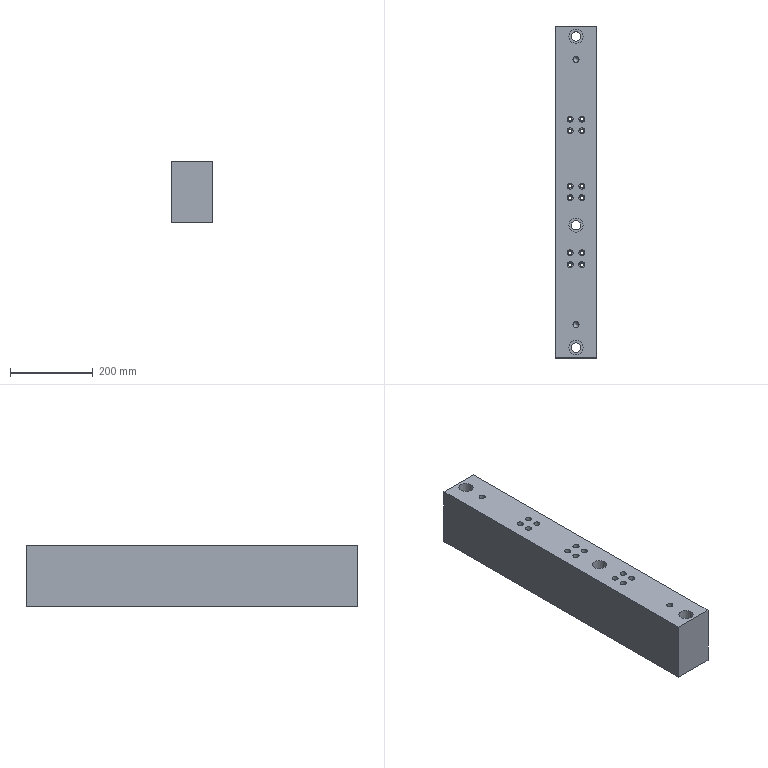Part | STEP file | lll_id2334_x_t | 1 solid | 61 faces | box 100 x 800 x 147.5 mm | volume 9817193 mm3 | cylinder 35 | plane 24 | cone 2 | commonest cylinder face diameters 9.009 x12 14.508 x12 23.009 x3 34.008 x3 80 x3 14.506 x2
STEP:
#1=CARTESIAN_POINT('',(2711.888,175.408,370.));
#2=VERTEX_POINT('',#1);
#3=CARTESIAN_POINT('',(2719.142,175.408,370.));
#4=DIRECTION('',(0.,0.,1.));
#5=DIRECTION('',(-1.,0.,0.));
#6=AXIS2_PLACEMENT_3D('',#3,#4,#5);
#7=CIRCLE('',#6,7.254);
#8=EDGE_CURVE('',#2,#2,#7,.T.);
#9=ORIENTED_EDGE('',*,*,#8,.F.);
#10=EDGE_LOOP('',(#9));
#11=FACE_BOUND('',#10,.T.);
#12=CARTESIAN_POINT('',(2711.888,147.124,370.));
#13=VERTEX_POINT('',#12);
#14=CARTESIAN_POINT('',(2719.142,147.124,370.));
#15=DIRECTION('',(0.,0.,1.));
#16=DIRECTION('',(-1.,0.,0.));
#17=AXIS2_PLACEMENT_3D('',#14,#15,#16);
#18=CIRCLE('',#17,7.254);
#19=EDGE_CURVE('',#13,#13,#18,.T.);
#20=ORIENTED_EDGE('',*,*,#19,.F.);
#21=EDGE_LOOP('',(#20));
#22=FACE_BOUND('',#21,.T.);
#23=CARTESIAN_POINT('',(2683.604,147.124,370.));
#24=VERTEX_POINT('',#23);
#25=CARTESIAN_POINT('',(2690.858,147.124,370.));
#26=DIRECTION('',(0.,0.,1.));
#27=DIRECTION('',(-1.,0.,0.));
#28=AXIS2_PLACEMENT_3D('',#25,#26,#27);
#29=CIRCLE('',#28,7.254);
#30=EDGE_CURVE('',#24,#24,#29,.T.);
#31=ORIENTED_EDGE('',*,*,#30,.F.);
#32=EDGE_LOOP('',(#31));
#33=FACE_BOUND('',#32,.T.);
#34=CARTESIAN_POINT('',(2683.604,14.142,370.));
#35=VERTEX_POINT('',#34);
#36=CARTESIAN_POINT('',(2690.858,14.142,370.));
#37=DIRECTION('',(0.,0.,1.));
#38=DIRECTION('',(-1.,0.,0.));
#39=AXIS2_PLACEMENT_3D('',#36,#37,#38);
#40=CIRCLE('',#39,7.254);
#41=EDGE_CURVE('',#35,#35,#40,.T.);
#42=ORIENTED_EDGE('',*,*,#41,.F.);
#43=EDGE_LOOP('',(#42));
#44=FACE_BOUND('',#43,.T.);
#45=CARTESIAN_POINT('',(2711.888,14.142,370.));
#46=VERTEX_POINT('',#45);
#47=CARTESIAN_POINT('',(2719.142,14.142,370.));
#48=DIRECTION('',(0.,0.,1.));
#49=DIRECTION('',(-1.,0.,0.));
#50=AXIS2_PLACEMENT_3D('',#47,#48,#49);
#51=CIRCLE('',#50,7.254);
#52=EDGE_CURVE('',#46,#46,#51,.T.);
#53=ORIENTED_EDGE('',*,*,#52,.F.);
#54=EDGE_LOOP('',(#53));
#55=FACE_BOUND('',#54,.T.);
#56=CARTESIAN_POINT('',(2711.888,-14.142,370.));
#57=VERTEX_POINT('',#56);
#58=CARTESIAN_POINT('',(2719.142,-14.142,370.));
#59=DIRECTION('',(0.,0.,1.));
#60=DIRECTION('',(-1.,0.,0.));
#61=AXIS2_PLACEMENT_3D('',#58,#59,#60);
#62=CIRCLE('',#61,7.254);
#63=EDGE_CURVE('',#57,#57,#62,.T.);
#64=ORIENTED_EDGE('',*,*,#63,.F.);
#65=EDGE_LOOP('',(#64));
#66=FACE_BOUND('',#65,.T.);
#67=CARTESIAN_POINT('',(2683.604,-14.142,370.));
#68=VERTEX_POINT('',#67);
#69=CARTESIAN_POINT('',(2690.858,-14.142,370.));
#70=DIRECTION('',(0.,0.,1.));
#71=DIRECTION('',(-1.,0.,0.));
#72=AXIS2_PLACEMENT_3D('',#69,#70,#71);
#73=CIRCLE('',#72,7.254);
#74=EDGE_CURVE('',#68,#68,#73,.T.);
#75=ORIENTED_EDGE('',*,*,#74,.F.);
#76=EDGE_LOOP('',(#75));
#77=FACE_BOUND('',#76,.T.);
#78=CARTESIAN_POINT('',(2711.888,-175.408,370.));
#79=VERTEX_POINT('',#78);
#80=CARTESIAN_POINT('',(2719.142,-175.408,370.));
#81=DIRECTION('',(0.,0.,1.));
#82=DIRECTION('',(-1.,0.,0.));
#83=AXIS2_PLACEMENT_3D('',#80,#81,#82);
#84=CIRCLE('',#83,7.254);
#85=EDGE_CURVE('',#79,#79,#84,.T.);
#86=ORIENTED_EDGE('',*,*,#85,.F.);
#87=EDGE_LOOP('',(#86));
#88=FACE_BOUND('',#87,.T.);
#89=CARTESIAN_POINT('',(2683.604,-175.408,370.));
#90=VERTEX_POINT('',#89);
#91=CARTESIAN_POINT('',(2690.858,-175.408,370.));
#92=DIRECTION('',(0.,0.,1.));
#93=DIRECTION('',(-1.,0.,0.));
#94=AXIS2_PLACEMENT_3D('',#91,#92,#93);
#95=CIRCLE('',#94,7.254);
#96=EDGE_CURVE('',#90,#90,#95,.T.);
#97=ORIENTED_EDGE('',*,*,#96,.F.);
#98=EDGE_LOOP('',(#97));
#99=FACE_BOUND('',#98,.T.);
#100=CARTESIAN_POINT('',(2683.604,-147.124,370.));
#101=VERTEX_POINT('',#100);
#102=CARTESIAN_POINT('',(2690.858,-147.124,370.));
#103=DIRECTION('',(0.,0.,1.));
#104=DIRECTION('',(-1.,0.,0.));
#105=AXIS2_PLACEMENT_3D('',#102,#103,#104);
#106=CIRCLE('',#105,7.254);
#107=EDGE_CURVE('',#101,#101,#106,.T.);
#108=ORIENTED_EDGE('',*,*,#107,.F.);
#109=EDGE_LOOP('',(#108));
#110=FACE_BOUND('',#109,.T.);
#111=CARTESIAN_POINT('',(2711.888,-147.124,370.));
#112=VERTEX_POINT('',#111);
#113=CARTESIAN_POINT('',(2719.142,-147.124,370.));
#114=DIRECTION('',(0.,0.,1.));
#115=DIRECTION('',(-1.,0.,0.));
#116=AXIS2_PLACEMENT_3D('',#113,#114,#115);
#117=CIRCLE('',#116,7.254);
#118=EDGE_CURVE('',#112,#112,#117,.T.);
#119=ORIENTED_EDGE('',*,*,#118,.F.);
#120=EDGE_LOOP('',(#119));
#121=FACE_BOUND('',#120,.T.);
#122=CARTESIAN_POINT('',(2683.604,175.408,370.));
#123=VERTEX_POINT('',#122);
#124=CARTESIAN_POINT('',(2690.858,175.408,370.));
#125=DIRECTION('',(0.,0.,1.));
#126=DIRECTION('',(-1.,0.,0.));
#127=AXIS2_PLACEMENT_3D('',#124,#125,#126);
#128=CIRCLE('',#127,7.254);
#129=EDGE_CURVE('',#123,#123,#128,.T.);
#130=ORIENTED_EDGE('',*,*,#129,.F.);
#131=EDGE_LOOP('',(#130));
#132=FACE_BOUND('',#131,.T.);
#133=CARTESIAN_POINT('',(2687.996,-80.,370.));
#134=VERTEX_POINT('',#133);
#135=CARTESIAN_POINT('',(2705.,-80.,370.));
#136=DIRECTION('',(0.,0.,-1.));
#137=DIRECTION('',(-1.,0.,0.));
#138=AXIS2_PLACEMENT_3D('',#135,#136,#137);
#139=CIRCLE('',#138,17.004);
#140=EDGE_CURVE('',#134,#134,#139,.T.);
#141=ORIENTED_EDGE('',*,*,#140,.T.);
#142=EDGE_LOOP('',(#141));
#143=FACE_BOUND('',#142,.T.);
#144=CARTESIAN_POINT('',(2755.,-400.,370.));
#145=VERTEX_POINT('',#144);
#146=CARTESIAN_POINT('',(2755.,400.,370.));
#147=VERTEX_POINT('',#146);
#148=CARTESIAN_POINT('',(2755.,600.,370.));
#149=DIRECTION('',(0.,1.,0.));
#150=VECTOR('',#149,1.);
#151=LINE('',#148,#150);
#152=EDGE_CURVE('',#145,#147,#151,.T.);
#153=ORIENTED_EDGE('',*,*,#152,.T.);
#154=CARTESIAN_POINT('',(2655.,400.,370.));
#155=VERTEX_POINT('',#154);
#156=CARTESIAN_POINT('',(2685.,400.,370.));
#157=DIRECTION('',(-1.,0.,0.));
#158=VECTOR('',#157,1.);
#159=LINE('',#156,#158);
#160=EDGE_CURVE('',#147,#155,#159,.T.);
#161=ORIENTED_EDGE('',*,*,#160,.T.);
#162=CARTESIAN_POINT('',(2655.,-400.,370.));
#163=VERTEX_POINT('',#162);
#164=CARTESIAN_POINT('',(2655.,0.,370.));
#165=DIRECTION('',(0.,1.,0.));
#166=VECTOR('',#165,1.);
#167=LINE('',#164,#166);
#168=EDGE_CURVE('',#163,#155,#167,.T.);
#169=ORIENTED_EDGE('',*,*,#168,.F.);
#170=CARTESIAN_POINT('',(2685.,-400.,370.));
#171=DIRECTION('',(1.,0.,0.));
#172=VECTOR('',#171,1.);
#173=LINE('',#170,#172);
#174=EDGE_CURVE('',#163,#145,#173,.T.);
#175=ORIENTED_EDGE('',*,*,#174,.T.);
#176=EDGE_LOOP('',(#153,#161,#169,#175));
#177=FACE_BOUND('',#176,.T.);
#178=CARTESIAN_POINT('',(2687.996,375.,370.));
#179=VERTEX_POINT('',#178);
#180=CARTESIAN_POINT('',(2705.,375.,370.));
#181=DIRECTION('',(0.,0.,-1.));
#182=DIRECTION('',(-1.,0.,0.));
#183=AXIS2_PLACEMENT_3D('',#180,#181,#182);
#184=CIRCLE('',#183,17.004);
#185=EDGE_CURVE('',#179,#179,#184,.T.);
#186=ORIENTED_EDGE('',*,*,#185,.T.);
#187=EDGE_LOOP('',(#186));
#188=FACE_BOUND('',#187,.T.);
#189=CARTESIAN_POINT('',(2687.996,-375.,370.));
#190=VERTEX_POINT('',#189);
#191=CARTESIAN_POINT('',(2705.,-375.,370.));
#192=DIRECTION('',(0.,0.,-1.));
#193=DIRECTION('',(-1.,0.,0.));
#194=AXIS2_PLACEMENT_3D('',#191,#192,#193);
#195=CIRCLE('',#194,17.004);
#196=EDGE_CURVE('',#190,#190,#195,.T.);
#197=ORIENTED_EDGE('',*,*,#196,.T.);
#198=EDGE_LOOP('',(#197));
#199=FACE_BOUND('',#198,.T.);
#200=CARTESIAN_POINT('',(2712.253,-320.,370.));
#201=VERTEX_POINT('',#200);
#202=CARTESIAN_POINT('',(2705.,-320.,370.));
#203=DIRECTION('',(0.,0.,-1.));
#204=DIRECTION('',(1.,0.,0.));
#205=AXIS2_PLACEMENT_3D('',#202,#203,#204);
#206=CIRCLE('',#205,7.253);
#207=EDGE_CURVE('',#201,#201,#206,.T.);
#208=ORIENTED_EDGE('',*,*,#207,.T.);
#209=EDGE_LOOP('',(#208));
#210=FACE_BOUND('',#209,.T.);
#211=CARTESIAN_POINT('',(2712.253,320.,370.));
#212=VERTEX_POINT('',#211);
#213=CARTESIAN_POINT('',(2705.,320.,370.));
#214=DIRECTION('',(0.,0.,1.));
#215=DIRECTION('',(1.,0.,0.));
#216=AXIS2_PLACEMENT_3D('',#213,#214,#215);
#217=CIRCLE('',#216,7.253);
#218=EDGE_CURVE('',#212,#212,#217,.T.);
#219=ORIENTED_EDGE('',*,*,#218,.F.);
#220=EDGE_LOOP('',(#219));
#221=FACE_BOUND('',#220,.T.);
#222=CARTESIAN_POINT('',(723.685,1.,370.));
#223=DIRECTION('',(0.,0.,-1.));
#224=DIRECTION('',(1.,0.,0.));
#225=AXIS2_PLACEMENT_3D('',#222,#223,#224);
#226=PLANE('',#225);
#227=ADVANCED_FACE('',(#11,#22,#33,#44,#55,#66,#77,#88,#99,#110,#121,#132,#143,#177,#188,#199,#210,#221),#226,.F.);
#228=CARTESIAN_POINT('',(2723.647,14.142,327.5));
#229=VERTEX_POINT('',#228);
#230=CARTESIAN_POINT('',(2719.142,14.142,327.5));
#231=DIRECTION('',(0.,0.,1.));
#232=DIRECTION('',(1.,0.,0.));
#233=AXIS2_PLACEMENT_3D('',#230,#231,#232);
#234=CIRCLE('',#233,4.505);
#235=EDGE_CURVE('',#229,#229,#234,.T.);
#236=ORIENTED_EDGE('',*,*,#235,.T.);
#237=EDGE_LOOP('',(#236));
#238=FACE_BOUND('',#237,.T.);
#239=CARTESIAN_POINT('',(2695.362,14.142,327.5));
#240=VERTEX_POINT('',#239);
#241=CARTESIAN_POINT('',(2690.858,14.142,327.5));
#242=DIRECTION('',(0.,0.,1.));
#243=DIRECTION('',(1.,0.,0.));
#244=AXIS2_PLACEMENT_3D('',#241,#242,#243);
#245=CIRCLE('',#244,4.505);
#246=EDGE_CURVE('',#240,#240,#245,.T.);
#247=ORIENTED_EDGE('',*,*,#246,.T.);
#248=EDGE_LOOP('',(#247));
#249=FACE_BOUND('',#248,.T.);
#250=CARTESIAN_POINT('',(2665.,0.,327.5));
#251=VERTEX_POINT('',#250);
#252=CARTESIAN_POINT('',(2705.,0.,327.5));
#253=DIRECTION('',(0.,0.,-1.));
#254=DIRECTION('',(-1.,0.,0.));
#255=AXIS2_PLACEMENT_3D('',#252,#253,#254);
#256=CIRCLE('',#255,40.);
#257=EDGE_CURVE('',#251,#251,#256,.T.);
#258=ORIENTED_EDGE('',*,*,#257,.T.);
#259=EDGE_LOOP('',(#258));
#260=FACE_BOUND('',#259,.T.);
#261=CARTESIAN_POINT('',(2695.362,-14.142,327.5));
#262=VERTEX_POINT('',#261);
#263=CARTESIAN_POINT('',(2690.858,-14.142,327.5));
#264=DIRECTION('',(0.,0.,1.));
#265=DIRECTION('',(1.,0.,0.));
#266=AXIS2_PLACEMENT_3D('',#263,#264,#265);
#267=CIRCLE('',#266,4.505);
#268=EDGE_CURVE('',#262,#262,#267,.T.);
#269=ORIENTED_EDGE('',*,*,#268,.T.);
#270=EDGE_LOOP('',(#269));
#271=FACE_BOUND('',#270,.T.);
#272=CARTESIAN_POINT('',(2723.647,-14.142,327.5));
#273=VERTEX_POINT('',#272);
#274=CARTESIAN_POINT('',(2719.142,-14.142,327.5));
#275=DIRECTION('',(0.,0.,1.));
#276=DIRECTION('',(1.,0.,0.));
#277=AXIS2_PLACEMENT_3D('',#274,#275,#276);
#278=CIRCLE('',#277,4.505);
#279=EDGE_CURVE('',#273,#273,#278,.T.);
#280=ORIENTED_EDGE('',*,*,#279,.T.);
#281=EDGE_LOOP('',(#280));
#282=FACE_BOUND('',#281,.T.);
#283=CARTESIAN_POINT('',(2705.,0.2078,327.5));
#284=DIRECTION('',(0.,0.,-1.));
#285=DIRECTION('',(-1.,0.,0.));
#286=AXIS2_PLACEMENT_3D('',#283,#284,#285);
#287=PLANE('',#286);
#288=ADVANCED_FACE('',(#238,#249,#260,#271,#282),#287,.T.);
#289=CARTESIAN_POINT('',(2723.647,-147.124,327.5));
#290=VERTEX_POINT('',#289);
#291=CARTESIAN_POINT('',(2719.142,-147.124,327.5));
#292=DIRECTION('',(0.,0.,1.));
#293=DIRECTION('',(1.,0.,0.));
#294=AXIS2_PLACEMENT_3D('',#291,#292,#293);
#295=CIRCLE('',#294,4.505);
#296=EDGE_CURVE('',#290,#290,#295,.T.);
#297=ORIENTED_EDGE('',*,*,#296,.T.);
#298=EDGE_LOOP('',(#297));
#299=FACE_BOUND('',#298,.T.);
#300=CARTESIAN_POINT('',(2695.362,-147.124,327.5));
#301=VERTEX_POINT('',#300);
#302=CARTESIAN_POINT('',(2690.858,-147.124,327.5));
#303=DIRECTION('',(0.,0.,1.));
#304=DIRECTION('',(1.,0.,0.));
#305=AXIS2_PLACEMENT_3D('',#302,#303,#304);
#306=CIRCLE('',#305,4.505);
#307=EDGE_CURVE('',#301,#301,#306,.T.);
#308=ORIENTED_EDGE('',*,*,#307,.T.);
#309=EDGE_LOOP('',(#308));
#310=FACE_BOUND('',#309,.T.);
#311=CARTESIAN_POINT('',(2665.,-161.266,327.5));
#312=VERTEX_POINT('',#311);
#313=CARTESIAN_POINT('',(2705.,-161.266,327.5));
#314=DIRECTION('',(0.,0.,-1.));
#315=DIRECTION('',(-1.,0.,0.));
#316=AXIS2_PLACEMENT_3D('',#313,#314,#315);
#317=CIRCLE('',#316,40.);
#318=EDGE_CURVE('',#312,#312,#317,.T.);
#319=ORIENTED_EDGE('',*,*,#318,.T.);
#320=EDGE_LOOP('',(#319));
#321=FACE_BOUND('',#320,.T.);
#322=CARTESIAN_POINT('',(2723.647,-175.408,327.5));
#323=VERTEX_POINT('',#322);
#324=CARTESIAN_POINT('',(2719.142,-175.408,327.5));
#325=DIRECTION('',(0.,0.,1.));
#326=DIRECTION('',(1.,0.,0.));
#327=AXIS2_PLACEMENT_3D('',#324,#325,#326);
#328=CIRCLE('',#327,4.505);
#329=EDGE_CURVE('',#323,#323,#328,.T.);
#330=ORIENTED_EDGE('',*,*,#329,.T.);
#331=EDGE_LOOP('',(#330));
#332=FACE_BOUND('',#331,.T.);
#333=CARTESIAN_POINT('',(2695.362,-175.408,327.5));
#334=VERTEX_POINT('',#333);
#335=CARTESIAN_POINT('',(2690.858,-175.408,327.5));
#336=DIRECTION('',(0.,0.,1.));
#337=DIRECTION('',(1.,0.,0.));
#338=AXIS2_PLACEMENT_3D('',#335,#336,#337);
#339=CIRCLE('',#338,4.505);
#340=EDGE_CURVE('',#334,#334,#339,.T.);
#341=ORIENTED_EDGE('',*,*,#340,.T.);
#342=EDGE_LOOP('',(#341));
#343=FACE_BOUND('',#342,.T.);
#344=CARTESIAN_POINT('',(2705.,-161.058,327.5));
#345=DIRECTION('',(0.,0.,-1.));
#346=DIRECTION('',(-1.,0.,0.));
#347=AXIS2_PLACEMENT_3D('',#344,#345,#346);
#348=PLANE('',#347);
#349=ADVANCED_FACE('',(#299,#310,#321,#332,#343),#348,.T.);
#350=CARTESIAN_POINT('',(2695.362,175.408,327.5));
#351=VERTEX_POINT('',#350);
#352=CARTESIAN_POINT('',(2690.858,175.408,327.5));
#353=DIRECTION('',(0.,0.,1.));
#354=DIRECTION('',(1.,0.,0.));
#355=AXIS2_PLACEMENT_3D('',#352,#353,#354);
#356=CIRCLE('',#355,4.505);
#357=EDGE_CURVE('',#351,#351,#356,.T.);
#358=ORIENTED_EDGE('',*,*,#357,.T.);
#359=EDGE_LOOP('',(#358));
#360=FACE_BOUND('',#359,.T.);
#361=CARTESIAN_POINT('',(2723.647,147.124,327.5));
#362=VERTEX_POINT('',#361);
#363=CARTESIAN_POINT('',(2719.142,147.124,327.5));
#364=DIRECTION('',(0.,0.,1.));
#365=DIRECTION('',(1.,0.,0.));
#366=AXIS2_PLACEMENT_3D('',#363,#364,#365);
#367=CIRCLE('',#366,4.505);
#368=EDGE_CURVE('',#362,#362,#367,.T.);
#369=ORIENTED_EDGE('',*,*,#368,.T.);
#370=EDGE_LOOP('',(#369));
#371=FACE_BOUND('',#370,.T.);
#372=CARTESIAN_POINT('',(2665.,161.266,327.5));
#373=VERTEX_POINT('',#372);
#374=CARTESIAN_POINT('',(2705.,161.266,327.5));
#375=DIRECTION('',(0.,0.,1.));
#376=DIRECTION('',(-1.,0.,0.));
#377=AXIS2_PLACEMENT_3D('',#374,#375,#376);
#378=CIRCLE('',#377,40.);
#379=EDGE_CURVE('',#373,#373,#378,.T.);
#380=ORIENTED_EDGE('',*,*,#379,.F.);
#381=EDGE_LOOP('',(#380));
#382=FACE_BOUND('',#381,.T.);
#383=CARTESIAN_POINT('',(2695.362,147.124,327.5));
#384=VERTEX_POINT('',#383);
#385=CARTESIAN_POINT('',(2690.858,147.124,327.5));
#386=DIRECTION('',(0.,0.,1.));
#387=DIRECTION('',(1.,0.,0.));
#388=AXIS2_PLACEMENT_3D('',#385,#386,#387);
#389=CIRCLE('',#388,4.505);
#390=EDGE_CURVE('',#384,#384,#389,.T.);
#391=ORIENTED_EDGE('',*,*,#390,.T.);
#392=EDGE_LOOP('',(#391));
#393=FACE_BOUND('',#392,.T.);
#394=CARTESIAN_POINT('',(2723.647,175.408,327.5));
#395=VERTEX_POINT('',#394);
#396=CARTESIAN_POINT('',(2719.142,175.408,327.5));
#397=DIRECTION('',(0.,0.,1.));
#398=DIRECTION('',(1.,0.,0.));
#399=AXIS2_PLACEMENT_3D('',#396,#397,#398);
#400=CIRCLE('',#399,4.505);
#401=EDGE_CURVE('',#395,#395,#400,.T.);
#402=ORIENTED_EDGE('',*,*,#401,.T.);
#403=EDGE_LOOP('',(#402));
#404=FACE_BOUND('',#403,.T.);
#405=CARTESIAN_POINT('',(2705.,161.474,327.5));
#406=DIRECTION('',(0.,0.,-1.));
#407=DIRECTION('',(-1.,0.,0.));
#408=AXIS2_PLACEMENT_3D('',#405,#406,#407);
#409=PLANE('',#408);
#410=ADVANCED_FACE('',(#360,#371,#382,#393,#404),#409,.T.);
#411=CARTESIAN_POINT('',(2693.495,-375.,222.5));
#412=VERTEX_POINT('',#411);
#413=CARTESIAN_POINT('',(2705.,-375.,222.5));
#414=DIRECTION('',(0.,0.,-1.));
#415=DIRECTION('',(-1.,0.,0.));
#416=AXIS2_PLACEMENT_3D('',#413,#414,#415);
#417=CIRCLE('',#416,11.505);
#418=EDGE_CURVE('',#412,#412,#417,.T.);
#419=ORIENTED_EDGE('',*,*,#418,.F.);
#420=EDGE_LOOP('',(#419));
#421=FACE_BOUND('',#420,.T.);
#422=CARTESIAN_POINT('',(2693.495,-80.,222.5));
#423=VERTEX_POINT('',#422);
#424=CARTESIAN_POINT('',(2705.,-80.,222.5));
#425=DIRECTION('',(0.,0.,-1.));
#426=DIRECTION('',(-1.,0.,0.));
#427=AXIS2_PLACEMENT_3D('',#424,#425,#426);
#428=CIRCLE('',#427,11.505);
#429=EDGE_CURVE('',#423,#423,#428,.T.);
#430=ORIENTED_EDGE('',*,*,#429,.F.);
#431=EDGE_LOOP('',(#430));
#432=FACE_BOUND('',#431,.T.);
#433=CARTESIAN_POINT('',(2693.495,375.,222.5));
#434=VERTEX_POINT('',#433);
#435=CARTESIAN_POINT('',(2705.,375.,222.5));
#436=DIRECTION('',(0.,0.,-1.));
#437=DIRECTION('',(-1.,0.,0.));
#438=AXIS2_PLACEMENT_3D('',#435,#436,#437);
#439=CIRCLE('',#438,11.505);
#440=EDGE_CURVE('',#434,#434,#439,.T.);
#441=ORIENTED_EDGE('',*,*,#440,.F.);
#442=EDGE_LOOP('',(#441));
#443=FACE_BOUND('',#442,.T.);
#444=CARTESIAN_POINT('',(2665.,-161.266,222.5));
#445=VERTEX_POINT('',#444);
#446=CARTESIAN_POINT('',(2705.,-161.266,222.5));
#447=DIRECTION('',(0.,0.,-1.));
#448=DIRECTION('',(-1.,0.,0.));
#449=AXIS2_PLACEMENT_3D('',#446,#447,#448);
#450=CIRCLE('',#449,40.);
#451=EDGE_CURVE('',#445,#445,#450,.T.);
#452=ORIENTED_EDGE('',*,*,#451,.F.);
#453=EDGE_LOOP('',(#452));
#454=FACE_BOUND('',#453,.T.);
#455=CARTESIAN_POINT('',(2665.,0.,222.5));
#456=VERTEX_POINT('',#455);
#457=CARTESIAN_POINT('',(2705.,0.,222.5));
#458=DIRECTION('',(0.,0.,-1.));
#459=DIRECTION('',(-1.,0.,0.));
#460=AXIS2_PLACEMENT_3D('',#457,#458,#459);
#461=CIRCLE('',#460,40.);
#462=EDGE_CURVE('',#456,#456,#461,.T.);
#463=ORIENTED_EDGE('',*,*,#462,.F.);
#464=EDGE_LOOP('',(#463));
#465=FACE_BOUND('',#464,.T.);
#466=CARTESIAN_POINT('',(2665.,161.266,222.5));
#467=VERTEX_POINT('',#466);
#468=CARTESIAN_POINT('',(2705.,161.266,222.5));
#469=DIRECTION('',(0.,0.,-1.));
#470=DIRECTION('',(-1.,0.,0.));
#471=AXIS2_PLACEMENT_3D('',#468,#469,#470);
#472=CIRCLE('',#471,40.);
#473=EDGE_CURVE('',#467,#467,#472,.T.);
#474=ORIENTED_EDGE('',*,*,#473,.F.);
#475=EDGE_LOOP('',(#474));
#476=FACE_BOUND('',#475,.T.);
#477=CARTESIAN_POINT('',(2755.,400.,222.5));
#478=VERTEX_POINT('',#477);
#479=CARTESIAN_POINT('',(2755.,-400.,222.5));
#480=VERTEX_POINT('',#479);
#481=CARTESIAN_POINT('',(2755.,1.,222.5));
#482=DIRECTION('',(0.,-1.,0.));
#483=VECTOR('',#482,1.);
#484=LINE('',#481,#483);
#485=EDGE_CURVE('',#478,#480,#484,.T.);
#486=ORIENTED_EDGE('',*,*,#485,.T.);
#487=CARTESIAN_POINT('',(2655.,-400.,222.5));
#488=VERTEX_POINT('',#487);
#489=CARTESIAN_POINT('',(4901.315,-400.,222.5));
#490=DIRECTION('',(-1.,0.,0.));
#491=VECTOR('',#490,1.);
#492=LINE('',#489,#491);
#493=EDGE_CURVE('',#480,#488,#492,.T.);
#494=ORIENTED_EDGE('',*,*,#493,.T.);
#495=CARTESIAN_POINT('',(2655.,400.,222.5));
#496=VERTEX_POINT('',#495);
#497=CARTESIAN_POINT('',(2655.,1.,222.5));
#498=DIRECTION('',(0.,-1.,0.));
#499=VECTOR('',#498,1.);
#500=LINE('',#497,#499);
#501=EDGE_CURVE('',#496,#488,#500,.T.);
#502=ORIENTED_EDGE('',*,*,#501,.F.);
#503=CARTESIAN_POINT('',(4901.315,400.,222.5));
#504=DIRECTION('',(1.,0.,0.));
#505=VECTOR('',#504,1.);
#506=LINE('',#503,#505);
#507=EDGE_CURVE('',#496,#478,#506,.T.);
#508=ORIENTED_EDGE('',*,*,#507,.T.);
#509=EDGE_LOOP('',(#486,#494,#502,#508));
#510=FACE_BOUND('',#509,.T.);
#511=CARTESIAN_POINT('',(4901.315,1.,222.5));
#512=DIRECTION('',(0.,0.,-1.));
#513=DIRECTION('',(-1.,0.,0.));
#514=AXIS2_PLACEMENT_3D('',#511,#512,#513);
#515=PLANE('',#514);
#516=ADVANCED_FACE('',(#421,#432,#443,#454,#465,#476,#510),#515,.T.);
#517=CARTESIAN_POINT('',(2755.,400.,291.25));
#518=DIRECTION('',(0.,0.,-1.));
#519=VECTOR('',#518,1.);
#520=LINE('',#517,#519);
#521=EDGE_CURVE('',#147,#478,#520,.T.);
#522=ORIENTED_EDGE('',*,*,#521,.F.);
#523=ORIENTED_EDGE('',*,*,#152,.F.);
#524=CARTESIAN_POINT('',(2755.,-400.,291.25));
#525=DIRECTION('',(0.,0.,1.));
#526=VECTOR('',#525,1.);
#527=LINE('',#524,#526);
#528=EDGE_CURVE('',#480,#145,#527,.T.);
#529=ORIENTED_EDGE('',*,*,#528,.F.);
#530=ORIENTED_EDGE('',*,*,#485,.F.);
#531=EDGE_LOOP('',(#522,#523,#529,#530));
#532=FACE_OUTER_BOUND('',#531,.T.);
#533=CARTESIAN_POINT('',(2755.,600.,360.));
#534=DIRECTION('',(1.,0.,0.));
#535=DIRECTION('',(0.,0.,-1.));
#536=AXIS2_PLACEMENT_3D('',#533,#534,#535);
#537=PLANE('',#536);
#538=ADVANCED_FACE('',(#532),#537,.T.);
#539=CARTESIAN_POINT('',(2655.,-400.,291.25));
#540=DIRECTION('',(0.,0.,-1.));
#541=VECTOR('',#540,1.);
#542=LINE('',#539,#541);
#543=EDGE_CURVE('',#163,#488,#542,.T.);
#544=ORIENTED_EDGE('',*,*,#543,.F.);
#545=ORIENTED_EDGE('',*,*,#168,.T.);
#546=CARTESIAN_POINT('',(2655.,400.,291.25));
#547=DIRECTION('',(0.,0.,-1.));
#548=VECTOR('',#547,1.);
#549=LINE('',#546,#548);
#550=EDGE_CURVE('',#155,#496,#549,.T.);
#551=ORIENTED_EDGE('',*,*,#550,.T.);
#552=ORIENTED_EDGE('',*,*,#501,.T.);
#553=EDGE_LOOP('',(#544,#545,#551,#552));
#554=FACE_OUTER_BOUND('',#553,.T.);
#555=CARTESIAN_POINT('',(2655.,0.,291.25));
#556=DIRECTION('',(1.,0.,0.));
#557=DIRECTION('',(0.,0.,-1.));
#558=AXIS2_PLACEMENT_3D('',#555,#556,#557);
#559=PLANE('',#558);
#560=ADVANCED_FACE('',(#554),#559,.F.);
#561=ORIENTED_EDGE('',*,*,#160,.F.);
#562=ORIENTED_EDGE('',*,*,#521,.T.);
#563=ORIENTED_EDGE('',*,*,#507,.F.);
#564=ORIENTED_EDGE('',*,*,#550,.F.);
#565=EDGE_LOOP('',(#561,#562,#563,#564));
#566=FACE_OUTER_BOUND('',#565,.T.);
#567=CARTESIAN_POINT('',(2685.,400.,291.25));
#568=DIRECTION('',(0.,1.,0.));
#569=DIRECTION('',(0.,0.,1.));
#570=AXIS2_PLACEMENT_3D('',#567,#568,#569);
#571=PLANE('',#570);
#572=ADVANCED_FACE('',(#566),#571,.T.);
#573=ORIENTED_EDGE('',*,*,#174,.F.);
#574=ORIENTED_EDGE('',*,*,#543,.T.);
#575=ORIENTED_EDGE('',*,*,#493,.F.);
#576=ORIENTED_EDGE('',*,*,#528,.T.);
#577=EDGE_LOOP('',(#573,#574,#575,#576));
#578=FACE_OUTER_BOUND('',#577,.T.);
#579=CARTESIAN_POINT('',(2685.,-400.,291.25));
#580=DIRECTION('',(0.,-1.,0.));
#581=DIRECTION('',(0.,0.,-1.));
#582=AXIS2_PLACEMENT_3D('',#579,#580,#581);
#583=PLANE('',#582);
#584=ADVANCED_FACE('',(#578),#583,.T.);
#585=ORIENTED_EDGE('',*,*,#379,.T.);
#586=EDGE_LOOP('',(#585));
#587=FACE_BOUND('',#586,.T.);
#588=ORIENTED_EDGE('',*,*,#473,.T.);
#589=EDGE_LOOP('',(#588));
#590=FACE_BOUND('',#589,.T.);
#591=CARTESIAN_POINT('',(2705.,161.266,346.5));
#592=DIRECTION('',(0.,0.,-1.));
#593=DIRECTION('',(1.,0.,0.));
#594=AXIS2_PLACEMENT_3D('',#591,#592,#593);
#595=CYLINDRICAL_SURFACE('',#594,40.);
#596=ADVANCED_FACE('',(#587,#590),#595,.F.);
#597=ORIENTED_EDGE('',*,*,#257,.F.);
#598=EDGE_LOOP('',(#597));
#599=FACE_BOUND('',#598,.T.);
#600=ORIENTED_EDGE('',*,*,#462,.T.);
#601=EDGE_LOOP('',(#600));
#602=FACE_BOUND('',#601,.T.);
#603=CARTESIAN_POINT('',(2705.,0.,181.5));
#604=DIRECTION('',(0.,0.,1.));
#605=DIRECTION('',(1.,0.,0.));
#606=AXIS2_PLACEMENT_3D('',#603,#604,#605);
#607=CYLINDRICAL_SURFACE('',#606,40.);
#608=ADVANCED_FACE('',(#599,#602),#607,.F.);
#609=ORIENTED_EDGE('',*,*,#318,.F.);
#610=EDGE_LOOP('',(#609));
#611=FACE_BOUND('',#610,.T.);
#612=ORIENTED_EDGE('',*,*,#451,.T.);
#613=EDGE_LOOP('',(#612));
#614=FACE_BOUND('',#613,.T.);
#615=CARTESIAN_POINT('',(2705.,-161.266,181.5));
#616=DIRECTION('',(0.,0.,1.));
#617=DIRECTION('',(1.,0.,0.));
#618=AXIS2_PLACEMENT_3D('',#615,#616,#617);
#619=CYLINDRICAL_SURFACE('',#618,40.);
#620=ADVANCED_FACE('',(#611,#614),#619,.F.);
#621=ORIENTED_EDGE('',*,*,#440,.T.);
#622=EDGE_LOOP('',(#621));
#623=FACE_BOUND('',#622,.T.);
#624=CARTESIAN_POINT('',(2693.495,375.,272.5));
#625=VERTEX_POINT('',#624);
#626=CARTESIAN_POINT('',(2705.,375.,272.5));
#627=DIRECTION('',(0.,0.,-1.));
#628=DIRECTION('',(-1.,0.,0.));
#629=AXIS2_PLACEMENT_3D('',#626,#627,#628);
#630=CIRCLE('',#629,11.505);
#631=EDGE_CURVE('',#625,#625,#630,.T.);
#632=ORIENTED_EDGE('',*,*,#631,.F.);
#633=EDGE_LOOP('',(#632));
#634=FACE_BOUND('',#633,.T.);
#635=CARTESIAN_POINT('',(2705.,375.,382.));
#636=DIRECTION('',(0.,0.,-1.));
#637=DIRECTION('',(1.,0.,0.));
#638=AXIS2_PLACEMENT_3D('',#635,#636,#637);
#639=CYLINDRICAL_SURFACE('',#638,11.505);
#640=ADVANCED_FACE('',(#623,#634),#639,.F.);
#641=ORIENTED_EDGE('',*,*,#631,.T.);
#642=EDGE_LOOP('',(#641));
#643=FACE_BOUND('',#642,.T.);
#644=CARTESIAN_POINT('',(2722.004,375.,272.5));
#645=VERTEX_POINT('',#644);
#646=CARTESIAN_POINT('',(2705.,375.,272.5));
#647=DIRECTION('',(0.,0.,-1.));
#648=DIRECTION('',(1.,0.,0.));
#649=AXIS2_PLACEMENT_3D('',#646,#647,#648);
#650=CIRCLE('',#649,17.004);
#651=EDGE_CURVE('',#645,#645,#650,.T.);
#652=ORIENTED_EDGE('',*,*,#651,.F.);
#653=EDGE_LOOP('',(#652));
#654=FACE_BOUND('',#653,.T.);
#655=CARTESIAN_POINT('',(2705.,375.,272.5));
#656=DIRECTION('',(0.,0.,-1.));
#657=DIRECTION('',(-1.,0.,0.));
#658=AXIS2_PLACEMENT_3D('',#655,#656,#657);
#659=PLANE('',#658);
#660=ADVANCED_FACE('',(#643,#654),#659,.F.);
#661=ORIENTED_EDGE('',*,*,#651,.T.);
#662=EDGE_LOOP('',(#661));
#663=FACE_BOUND('',#662,.T.);
#664=ORIENTED_EDGE('',*,*,#185,.F.);
#665=EDGE_LOOP('',(#664));
#666=FACE_BOUND('',#665,.T.);
#667=CARTESIAN_POINT('',(2705.,375.,380.));
#668=DIRECTION('',(0.,0.,-1.));
#669=DIRECTION('',(1.,0.,0.));
#670=AXIS2_PLACEMENT_3D('',#667,#668,#669);
#671=CYLINDRICAL_SURFACE('',#670,17.004);
#672=ADVANCED_FACE('',(#663,#666),#671,.F.);
#673=ORIENTED_EDGE('',*,*,#429,.T.);
#674=EDGE_LOOP('',(#673));
#675=FACE_BOUND('',#674,.T.);
#676=CARTESIAN_POINT('',(2693.495,-80.,272.5));
#677=VERTEX_POINT('',#676);
#678=CARTESIAN_POINT('',(2705.,-80.,272.5));
#679=DIRECTION('',(0.,0.,-1.));
#680=DIRECTION('',(-1.,0.,0.));
#681=AXIS2_PLACEMENT_3D('',#678,#679,#680);
#682=CIRCLE('',#681,11.505);
#683=EDGE_CURVE('',#677,#677,#682,.T.);
#684=ORIENTED_EDGE('',*,*,#683,.F.);
#685=EDGE_LOOP('',(#684));
#686=FACE_BOUND('',#685,.T.);
#687=CARTESIAN_POINT('',(2705.,-80.,382.));
#688=DIRECTION('',(0.,0.,-1.));
#689=DIRECTION('',(1.,0.,0.));
#690=AXIS2_PLACEMENT_3D('',#687,#688,#689);
#691=CYLINDRICAL_SURFACE('',#690,11.505);
#692=ADVANCED_FACE('',(#675,#686),#691,.F.);
#693=ORIENTED_EDGE('',*,*,#683,.T.);
#694=EDGE_LOOP('',(#693));
#695=FACE_BOUND('',#694,.T.);
#696=CARTESIAN_POINT('',(2722.004,-80.,272.5));
#697=VERTEX_POINT('',#696);
#698=CARTESIAN_POINT('',(2705.,-80.,272.5));
#699=DIRECTION('',(0.,0.,-1.));
#700=DIRECTION('',(1.,0.,0.));
#701=AXIS2_PLACEMENT_3D('',#698,#699,#700);
#702=CIRCLE('',#701,17.004);
#703=EDGE_CURVE('',#697,#697,#702,.T.);
#704=ORIENTED_EDGE('',*,*,#703,.F.);
#705=EDGE_LOOP('',(#704));
#706=FACE_BOUND('',#705,.T.);
#707=CARTESIAN_POINT('',(2705.,-80.,272.5));
#708=DIRECTION('',(0.,0.,-1.));
#709=DIRECTION('',(-1.,0.,0.));
#710=AXIS2_PLACEMENT_3D('',#707,#708,#709);
#711=PLANE('',#710);
#712=ADVANCED_FACE('',(#695,#706),#711,.F.);
#713=ORIENTED_EDGE('',*,*,#703,.T.);
#714=EDGE_LOOP('',(#713));
#715=FACE_BOUND('',#714,.T.);
#716=ORIENTED_EDGE('',*,*,#140,.F.);
#717=EDGE_LOOP('',(#716));
#718=FACE_BOUND('',#717,.T.);
#719=CARTESIAN_POINT('',(2705.,-80.,380.));
#720=DIRECTION('',(0.,0.,-1.));
#721=DIRECTION('',(1.,0.,0.));
#722=AXIS2_PLACEMENT_3D('',#719,#720,#721);
#723=CYLINDRICAL_SURFACE('',#722,17.004);
#724=ADVANCED_FACE('',(#715,#718),#723,.F.);
#725=ORIENTED_EDGE('',*,*,#418,.T.);
#726=EDGE_LOOP('',(#725));
#727=FACE_BOUND('',#726,.T.);
#728=CARTESIAN_POINT('',(2693.495,-375.,272.5));
#729=VERTEX_POINT('',#728);
#730=CARTESIAN_POINT('',(2705.,-375.,272.5));
#731=DIRECTION('',(0.,0.,-1.));
#732=DIRECTION('',(-1.,0.,0.));
#733=AXIS2_PLACEMENT_3D('',#730,#731,#732);
#734=CIRCLE('',#733,11.505);
#735=EDGE_CURVE('',#729,#729,#734,.T.);
#736=ORIENTED_EDGE('',*,*,#735,.F.);
#737=EDGE_LOOP('',(#736));
#738=FACE_BOUND('',#737,.T.);
#739=CARTESIAN_POINT('',(2705.,-375.,382.));
#740=DIRECTION('',(0.,0.,-1.));
#741=DIRECTION('',(1.,0.,0.));
#742=AXIS2_PLACEMENT_3D('',#739,#740,#741);
#743=CYLINDRICAL_SURFACE('',#742,11.505);
#744=ADVANCED_FACE('',(#727,#738),#743,.F.);
#745=ORIENTED_EDGE('',*,*,#735,.T.);
#746=EDGE_LOOP('',(#745));
#747=FACE_BOUND('',#746,.T.);
#748=CARTESIAN_POINT('',(2722.004,-375.,272.5));
#749=VERTEX_POINT('',#748);
#750=CARTESIAN_POINT('',(2705.,-375.,272.5));
#751=DIRECTION('',(0.,0.,-1.));
#752=DIRECTION('',(1.,0.,0.));
#753=AXIS2_PLACEMENT_3D('',#750,#751,#752);
#754=CIRCLE('',#753,17.004);
#755=EDGE_CURVE('',#749,#749,#754,.T.);
#756=ORIENTED_EDGE('',*,*,#755,.F.);
#757=EDGE_LOOP('',(#756));
#758=FACE_BOUND('',#757,.T.);
#759=CARTESIAN_POINT('',(2705.,-375.,272.5));
#760=DIRECTION('',(0.,0.,-1.));
#761=DIRECTION('',(-1.,0.,0.));
#762=AXIS2_PLACEMENT_3D('',#759,#760,#761);
#763=PLANE('',#762);
#764=ADVANCED_FACE('',(#747,#758),#763,.F.);
#765=ORIENTED_EDGE('',*,*,#755,.T.);
#766=EDGE_LOOP('',(#765));
#767=FACE_BOUND('',#766,.T.);
#768=ORIENTED_EDGE('',*,*,#196,.F.);
#769=EDGE_LOOP('',(#768));
#770=FACE_BOUND('',#769,.T.);
#771=CARTESIAN_POINT('',(2705.,-375.,380.));
#772=DIRECTION('',(0.,0.,-1.));
#773=DIRECTION('',(1.,0.,0.));
#774=AXIS2_PLACEMENT_3D('',#771,#772,#773);
#775=CYLINDRICAL_SURFACE('',#774,17.004);
#776=ADVANCED_FACE('',(#767,#770),#775,.F.);
#777=CARTESIAN_POINT('',(2726.396,147.124,349.));
#778=VERTEX_POINT('',#777);
#779=CARTESIAN_POINT('',(2719.142,147.124,349.));
#780=DIRECTION('',(0.,0.,-1.));
#781=DIRECTION('',(1.,0.,0.));
#782=AXIS2_PLACEMENT_3D('',#779,#780,#781);
#783=CIRCLE('',#782,7.254);
#784=EDGE_CURVE('',#778,#778,#783,.T.);
#785=ORIENTED_EDGE('',*,*,#784,.T.);
#786=EDGE_LOOP('',(#785));
#787=FACE_BOUND('',#786,.T.);
#788=ORIENTED_EDGE('',*,*,#19,.T.);
#789=EDGE_LOOP('',(#788));
#790=FACE_BOUND('',#789,.T.);
#791=CARTESIAN_POINT('',(2719.142,147.124,360.));
#792=DIRECTION('',(0.,0.,-1.));
#793=DIRECTION('',(1.,0.,0.));
#794=AXIS2_PLACEMENT_3D('',#791,#792,#793);
#795=CYLINDRICAL_SURFACE('',#794,7.254);
#796=ADVANCED_FACE('',(#787,#790),#795,.F.);
#797=CARTESIAN_POINT('',(2714.638,147.124,349.));
#798=VERTEX_POINT('',#797);
#799=CARTESIAN_POINT('',(2719.142,147.124,349.));
#800=DIRECTION('',(0.,0.,-1.));
#801=DIRECTION('',(-1.,0.,0.));
#802=AXIS2_PLACEMENT_3D('',#799,#800,#801);
#803=CIRCLE('',#802,4.505);
#804=EDGE_CURVE('',#798,#798,#803,.T.);
#805=ORIENTED_EDGE('',*,*,#804,.T.);
#806=EDGE_LOOP('',(#805));
#807=FACE_BOUND('',#806,.T.);
#808=ORIENTED_EDGE('',*,*,#784,.F.);
#809=EDGE_LOOP('',(#808));
#810=FACE_BOUND('',#809,.T.);
#811=CARTESIAN_POINT('',(2719.142,147.124,349.));
#812=DIRECTION('',(0.,0.,-1.));
#813=DIRECTION('',(-1.,0.,0.));
#814=AXIS2_PLACEMENT_3D('',#811,#812,#813);
#815=PLANE('',#814);
#816=ADVANCED_FACE('',(#807,#810),#815,.F.);
#817=ORIENTED_EDGE('',*,*,#804,.F.);
#818=EDGE_LOOP('',(#817));
#819=FACE_BOUND('',#818,.T.);
#820=ORIENTED_EDGE('',*,*,#368,.F.);
#821=EDGE_LOOP('',(#820));
#822=FACE_BOUND('',#821,.T.);
#823=CARTESIAN_POINT('',(2719.142,147.124,360.));
#824=DIRECTION('',(0.,0.,-1.));
#825=DIRECTION('',(1.,0.,0.));
#826=AXIS2_PLACEMENT_3D('',#823,#824,#825);
#827=CYLINDRICAL_SURFACE('',#826,4.505);
#828=ADVANCED_FACE('',(#819,#822),#827,.F.);
#829=CARTESIAN_POINT('',(2698.112,147.124,349.));
#830=VERTEX_POINT('',#829);
#831=CARTESIAN_POINT('',(2690.858,147.124,349.));
#832=DIRECTION('',(0.,0.,-1.));
#833=DIRECTION('',(1.,0.,0.));
#834=AXIS2_PLACEMENT_3D('',#831,#832,#833);
#835=CIRCLE('',#834,7.254);
#836=EDGE_CURVE('',#830,#830,#835,.T.);
#837=ORIENTED_EDGE('',*,*,#836,.T.);
#838=EDGE_LOOP('',(#837));
#839=FACE_BOUND('',#838,.T.);
#840=ORIENTED_EDGE('',*,*,#30,.T.);
#841=EDGE_LOOP('',(#840));
#842=FACE_BOUND('',#841,.T.);
#843=CARTESIAN_POINT('',(2690.858,147.124,360.));
#844=DIRECTION('',(0.,0.,-1.));
#845=DIRECTION('',(1.,0.,0.));
#846=AXIS2_PLACEMENT_3D('',#843,#844,#845);
#847=CYLINDRICAL_SURFACE('',#846,7.254);
#848=ADVANCED_FACE('',(#839,#842),#847,.F.);
#849=CARTESIAN_POINT('',(2686.353,147.124,349.));
#850=VERTEX_POINT('',#849);
#851=CARTESIAN_POINT('',(2690.858,147.124,349.));
#852=DIRECTION('',(0.,0.,-1.));
#853=DIRECTION('',(-1.,0.,0.));
#854=AXIS2_PLACEMENT_3D('',#851,#852,#853);
#855=CIRCLE('',#854,4.505);
#856=EDGE_CURVE('',#850,#850,#855,.T.);
#857=ORIENTED_EDGE('',*,*,#856,.F.);
#858=EDGE_LOOP('',(#857));
#859=FACE_BOUND('',#858,.T.);
#860=ORIENTED_EDGE('',*,*,#390,.F.);
#861=EDGE_LOOP('',(#860));
#862=FACE_BOUND('',#861,.T.);
#863=CARTESIAN_POINT('',(2690.858,147.124,360.));
#864=DIRECTION('',(0.,0.,-1.));
#865=DIRECTION('',(1.,0.,0.));
#866=AXIS2_PLACEMENT_3D('',#863,#864,#865);
#867=CYLINDRICAL_SURFACE('',#866,4.505);
#868=ADVANCED_FACE('',(#859,#862),#867,.F.);
#869=ORIENTED_EDGE('',*,*,#856,.T.);
#870=EDGE_LOOP('',(#869));
#871=FACE_BOUND('',#870,.T.);
#872=ORIENTED_EDGE('',*,*,#836,.F.);
#873=EDGE_LOOP('',(#872));
#874=FACE_BOUND('',#873,.T.);
#875=CARTESIAN_POINT('',(2690.858,147.124,349.));
#876=DIRECTION('',(0.,0.,-1.));
#877=DIRECTION('',(-1.,0.,0.));
#878=AXIS2_PLACEMENT_3D('',#875,#876,#877);
#879=PLANE('',#878);
#880=ADVANCED_FACE('',(#871,#874),#879,.F.);
#881=CARTESIAN_POINT('',(2698.112,14.142,349.));
#882=VERTEX_POINT('',#881);
#883=CARTESIAN_POINT('',(2690.858,14.142,349.));
#884=DIRECTION('',(0.,0.,-1.));
#885=DIRECTION('',(1.,0.,0.));
#886=AXIS2_PLACEMENT_3D('',#883,#884,#885);
#887=CIRCLE('',#886,7.254);
#888=EDGE_CURVE('',#882,#882,#887,.T.);
#889=ORIENTED_EDGE('',*,*,#888,.T.);
#890=EDGE_LOOP('',(#889));
#891=FACE_BOUND('',#890,.T.);
#892=ORIENTED_EDGE('',*,*,#41,.T.);
#893=EDGE_LOOP('',(#892));
#894=FACE_BOUND('',#893,.T.);
#895=CARTESIAN_POINT('',(2690.858,14.142,360.));
#896=DIRECTION('',(0.,0.,-1.));
#897=DIRECTION('',(1.,0.,0.));
#898=AXIS2_PLACEMENT_3D('',#895,#896,#897);
#899=CYLINDRICAL_SURFACE('',#898,7.254);
#900=ADVANCED_FACE('',(#891,#894),#899,.F.);
#901=CARTESIAN_POINT('',(2686.353,14.142,349.));
#902=VERTEX_POINT('',#901);
#903=CARTESIAN_POINT('',(2690.858,14.142,349.));
#904=DIRECTION('',(0.,0.,-1.));
#905=DIRECTION('',(-1.,0.,0.));
#906=AXIS2_PLACEMENT_3D('',#903,#904,#905);
#907=CIRCLE('',#906,4.505);
#908=EDGE_CURVE('',#902,#902,#907,.T.);
#909=ORIENTED_EDGE('',*,*,#908,.T.);
#910=EDGE_LOOP('',(#909));
#911=FACE_BOUND('',#910,.T.);
#912=ORIENTED_EDGE('',*,*,#888,.F.);
#913=EDGE_LOOP('',(#912));
#914=FACE_BOUND('',#913,.T.);
#915=CARTESIAN_POINT('',(2690.858,14.142,349.));
#916=DIRECTION('',(0.,0.,-1.));
#917=DIRECTION('',(-1.,0.,0.));
#918=AXIS2_PLACEMENT_3D('',#915,#916,#917);
#919=PLANE('',#918);
#920=ADVANCED_FACE('',(#911,#914),#919,.F.);
#921=ORIENTED_EDGE('',*,*,#908,.F.);
#922=EDGE_LOOP('',(#921));
#923=FACE_BOUND('',#922,.T.);
#924=ORIENTED_EDGE('',*,*,#246,.F.);
#925=EDGE_LOOP('',(#924));
#926=FACE_BOUND('',#925,.T.);
#927=CARTESIAN_POINT('',(2690.858,14.142,360.));
#928=DIRECTION('',(0.,0.,-1.));
#929=DIRECTION('',(1.,0.,0.));
#930=AXIS2_PLACEMENT_3D('',#927,#928,#929);
#931=CYLINDRICAL_SURFACE('',#930,4.505);
#932=ADVANCED_FACE('',(#923,#926),#931,.F.);
#933=CARTESIAN_POINT('',(2698.112,175.408,349.));
#934=VERTEX_POINT('',#933);
#935=CARTESIAN_POINT('',(2690.858,175.408,349.));
#936=DIRECTION('',(0.,0.,-1.));
#937=DIRECTION('',(1.,0.,0.));
#938=AXIS2_PLACEMENT_3D('',#935,#936,#937);
#939=CIRCLE('',#938,7.254);
#940=EDGE_CURVE('',#934,#934,#939,.T.);
#941=ORIENTED_EDGE('',*,*,#940,.T.);
#942=EDGE_LOOP('',(#941));
#943=FACE_BOUND('',#942,.T.);
#944=ORIENTED_EDGE('',*,*,#129,.T.);
#945=EDGE_LOOP('',(#944));
#946=FACE_BOUND('',#945,.T.);
#947=CARTESIAN_POINT('',(2690.858,175.408,360.));
#948=DIRECTION('',(0.,0.,-1.));
#949=DIRECTION('',(1.,0.,0.));
#950=AXIS2_PLACEMENT_3D('',#947,#948,#949);
#951=CYLINDRICAL_SURFACE('',#950,7.254);
#952=ADVANCED_FACE('',(#943,#946),#951,.F.);
#953=CARTESIAN_POINT('',(2686.353,175.408,349.));
#954=VERTEX_POINT('',#953);
#955=CARTESIAN_POINT('',(2690.858,175.408,349.));
#956=DIRECTION('',(0.,0.,-1.));
#957=DIRECTION('',(-1.,0.,0.));
#958=AXIS2_PLACEMENT_3D('',#955,#956,#957);
#959=CIRCLE('',#958,4.505);
#960=EDGE_CURVE('',#954,#954,#959,.T.);
#961=ORIENTED_EDGE('',*,*,#960,.T.);
#962=EDGE_LOOP('',(#961));
#963=FACE_BOUND('',#962,.T.);
#964=ORIENTED_EDGE('',*,*,#940,.F.);
#965=EDGE_LOOP('',(#964));
#966=FACE_BOUND('',#965,.T.);
#967=CARTESIAN_POINT('',(2690.858,175.408,349.));
#968=DIRECTION('',(0.,0.,-1.));
#969=DIRECTION('',(-1.,0.,0.));
#970=AXIS2_PLACEMENT_3D('',#967,#968,#969);
#971=PLANE('',#970);
#972=ADVANCED_FACE('',(#963,#966),#971,.F.);
#973=ORIENTED_EDGE('',*,*,#960,.F.);
#974=EDGE_LOOP('',(#973));
#975=FACE_BOUND('',#974,.T.);
#976=ORIENTED_EDGE('',*,*,#357,.F.);
#977=EDGE_LOOP('',(#976));
#978=FACE_BOUND('',#977,.T.);
#979=CARTESIAN_POINT('',(2690.858,175.408,360.));
#980=DIRECTION('',(0.,0.,-1.));
#981=DIRECTION('',(1.,0.,0.));
#982=AXIS2_PLACEMENT_3D('',#979,#980,#981);
#983=CYLINDRICAL_SURFACE('',#982,4.505);
#984=ADVANCED_FACE('',(#975,#978),#983,.F.);
#985=CARTESIAN_POINT('',(2726.396,175.408,349.));
#986=VERTEX_POINT('',#985);
#987=CARTESIAN_POINT('',(2719.142,175.408,349.));
#988=DIRECTION('',(0.,0.,-1.));
#989=DIRECTION('',(1.,0.,0.));
#990=AXIS2_PLACEMENT_3D('',#987,#988,#989);
#991=CIRCLE('',#990,7.254);
#992=EDGE_CURVE('',#986,#986,#991,.T.);
#993=ORIENTED_EDGE('',*,*,#992,.T.);
#994=EDGE_LOOP('',(#993));
#995=FACE_BOUND('',#994,.T.);
#996=ORIENTED_EDGE('',*,*,#8,.T.);
#997=EDGE_LOOP('',(#996));
#998=FACE_BOUND('',#997,.T.);
#999=CARTESIAN_POINT('',(2719.142,175.408,360.));
#1000=DIRECTION('',(0.,0.,-1.));
#1001=DIRECTION('',(1.,0.,0.));
#1002=AXIS2_PLACEMENT_3D('',#999,#1000,#1001);
#1003=CYLINDRICAL_SURFACE('',#1002,7.254);
#1004=ADVANCED_FACE('',(#995,#998),#1003,.F.);
#1005=CARTESIAN_POINT('',(2714.638,175.408,349.));
#1006=VERTEX_POINT('',#1005);
#1007=CARTESIAN_POINT('',(2719.142,175.408,349.));
#1008=DIRECTION('',(0.,0.,-1.));
#1009=DIRECTION('',(-1.,0.,0.));
#1010=AXIS2_PLACEMENT_3D('',#1007,#1008,#1009);
#1011=CIRCLE('',#1010,4.505);
#1012=EDGE_CURVE('',#1006,#1006,#1011,.T.);
#1013=ORIENTED_EDGE('',*,*,#1012,.T.);
#1014=EDGE_LOOP('',(#1013));
#1015=FACE_BOUND('',#1014,.T.);
#1016=ORIENTED_EDGE('',*,*,#992,.F.);
#1017=EDGE_LOOP('',(#1016));
#1018=FACE_BOUND('',#1017,.T.);
#1019=CARTESIAN_POINT('',(2719.142,175.408,349.));
#1020=DIRECTION('',(0.,0.,-1.));
#1021=DIRECTION('',(-1.,0.,0.));
#1022=AXIS2_PLACEMENT_3D('',#1019,#1020,#1021);
#1023=PLANE('',#1022);
#1024=ADVANCED_FACE('',(#1015,#1018),#1023,.F.);
#1025=ORIENTED_EDGE('',*,*,#1012,.F.);
#1026=EDGE_LOOP('',(#1025));
#1027=FACE_BOUND('',#1026,.T.);
#1028=ORIENTED_EDGE('',*,*,#401,.F.);
#1029=EDGE_LOOP('',(#1028));
#1030=FACE_BOUND('',#1029,.T.);
#1031=CARTESIAN_POINT('',(2719.142,175.408,360.));
#1032=DIRECTION('',(0.,0.,-1.));
#1033=DIRECTION('',(1.,0.,0.));
#1034=AXIS2_PLACEMENT_3D('',#1031,#1032,#1033);
#1035=CYLINDRICAL_SURFACE('',#1034,4.505);
#1036=ADVANCED_FACE('',(#1027,#1030),#1035,.F.);
#1037=CARTESIAN_POINT('',(2698.112,-14.142,349.));
#1038=VERTEX_POINT('',#1037);
#1039=CARTESIAN_POINT('',(2690.858,-14.142,349.));
#1040=DIRECTION('',(0.,0.,-1.));
#1041=DIRECTION('',(1.,0.,0.));
#1042=AXIS2_PLACEMENT_3D('',#1039,#1040,#1041);
#1043=CIRCLE('',#1042,7.254);
#1044=EDGE_CURVE('',#1038,#1038,#1043,.T.);
#1045=ORIENTED_EDGE('',*,*,#1044,.T.);
#1046=EDGE_LOOP('',(#1045));
#1047=FACE_BOUND('',#1046,.T.);
#1048=ORIENTED_EDGE('',*,*,#74,.T.);
#1049=EDGE_LOOP('',(#1048));
#1050=FACE_BOUND('',#1049,.T.);
#1051=CARTESIAN_POINT('',(2690.858,-14.142,360.));
#1052=DIRECTION('',(0.,0.,-1.));
#1053=DIRECTION('',(1.,0.,0.));
#1054=AXIS2_PLACEMENT_3D('',#1051,#1052,#1053);
#1055=CYLINDRICAL_SURFACE('',#1054,7.254);
#1056=ADVANCED_FACE('',(#1047,#1050),#1055,.F.);
#1057=CARTESIAN_POINT('',(2686.353,-14.142,349.));
#1058=VERTEX_POINT('',#1057);
#1059=CARTESIAN_POINT('',(2690.858,-14.142,349.));
#1060=DIRECTION('',(0.,0.,-1.));
#1061=DIRECTION('',(-1.,0.,0.));
#1062=AXIS2_PLACEMENT_3D('',#1059,#1060,#1061);
#1063=CIRCLE('',#1062,4.505);
#1064=EDGE_CURVE('',#1058,#1058,#1063,.T.);
#1065=ORIENTED_EDGE('',*,*,#1064,.F.);
#1066=EDGE_LOOP('',(#1065));
#1067=FACE_BOUND('',#1066,.T.);
#1068=ORIENTED_EDGE('',*,*,#268,.F.);
#1069=EDGE_LOOP('',(#1068));
#1070=FACE_BOUND('',#1069,.T.);
#1071=CARTESIAN_POINT('',(2690.858,-14.142,360.));
#1072=DIRECTION('',(0.,0.,-1.));
#1073=DIRECTION('',(1.,0.,0.));
#1074=AXIS2_PLACEMENT_3D('',#1071,#1072,#1073);
#1075=CYLINDRICAL_SURFACE('',#1074,4.505);
#1076=ADVANCED_FACE('',(#1067,#1070),#1075,.F.);
#1077=ORIENTED_EDGE('',*,*,#1064,.T.);
#1078=EDGE_LOOP('',(#1077));
#1079=FACE_BOUND('',#1078,.T.);
#1080=ORIENTED_EDGE('',*,*,#1044,.F.);
#1081=EDGE_LOOP('',(#1080));
#1082=FACE_BOUND('',#1081,.T.);
#1083=CARTESIAN_POINT('',(2690.858,-14.142,349.));
#1084=DIRECTION('',(0.,0.,-1.));
#1085=DIRECTION('',(-1.,0.,0.));
#1086=AXIS2_PLACEMENT_3D('',#1083,#1084,#1085);
#1087=PLANE('',#1086);
#1088=ADVANCED_FACE('',(#1079,#1082),#1087,.F.);
#1089=CARTESIAN_POINT('',(2698.112,-147.124,349.));
#1090=VERTEX_POINT('',#1089);
#1091=CARTESIAN_POINT('',(2690.858,-147.124,349.));
#1092=DIRECTION('',(0.,0.,-1.));
#1093=DIRECTION('',(1.,0.,0.));
#1094=AXIS2_PLACEMENT_3D('',#1091,#1092,#1093);
#1095=CIRCLE('',#1094,7.254);
#1096=EDGE_CURVE('',#1090,#1090,#1095,.T.);
#1097=ORIENTED_EDGE('',*,*,#1096,.T.);
#1098=EDGE_LOOP('',(#1097));
#1099=FACE_BOUND('',#1098,.T.);
#1100=ORIENTED_EDGE('',*,*,#107,.T.);
#1101=EDGE_LOOP('',(#1100));
#1102=FACE_BOUND('',#1101,.T.);
#1103=CARTESIAN_POINT('',(2690.858,-147.124,360.));
#1104=DIRECTION('',(0.,0.,-1.));
#1105=DIRECTION('',(1.,0.,0.));
#1106=AXIS2_PLACEMENT_3D('',#1103,#1104,#1105);
#1107=CYLINDRICAL_SURFACE('',#1106,7.254);
#1108=ADVANCED_FACE('',(#1099,#1102),#1107,.F.);
#1109=CARTESIAN_POINT('',(2686.353,-147.124,349.));
#1110=VERTEX_POINT('',#1109);
#1111=CARTESIAN_POINT('',(2690.858,-147.124,349.));
#1112=DIRECTION('',(0.,0.,-1.));
#1113=DIRECTION('',(-1.,0.,0.));
#1114=AXIS2_PLACEMENT_3D('',#1111,#1112,#1113);
#1115=CIRCLE('',#1114,4.505);
#1116=EDGE_CURVE('',#1110,#1110,#1115,.T.);
#1117=ORIENTED_EDGE('',*,*,#1116,.T.);
#1118=EDGE_LOOP('',(#1117));
#1119=FACE_BOUND('',#1118,.T.);
#1120=ORIENTED_EDGE('',*,*,#1096,.F.);
#1121=EDGE_LOOP('',(#1120));
#1122=FACE_BOUND('',#1121,.T.);
#1123=CARTESIAN_POINT('',(2690.858,-147.124,349.));
#1124=DIRECTION('',(0.,0.,-1.));
#1125=DIRECTION('',(-1.,0.,0.));
#1126=AXIS2_PLACEMENT_3D('',#1123,#1124,#1125);
#1127=PLANE('',#1126);
#1128=ADVANCED_FACE('',(#1119,#1122),#1127,.F.);
#1129=ORIENTED_EDGE('',*,*,#1116,.F.);
#1130=EDGE_LOOP('',(#1129));
#1131=FACE_BOUND('',#1130,.T.);
#1132=ORIENTED_EDGE('',*,*,#307,.F.);
#1133=EDGE_LOOP('',(#1132));
#1134=FACE_BOUND('',#1133,.T.);
#1135=CARTESIAN_POINT('',(2690.858,-147.124,360.));
#1136=DIRECTION('',(0.,0.,-1.));
#1137=DIRECTION('',(1.,0.,0.));
#1138=AXIS2_PLACEMENT_3D('',#1135,#1136,#1137);
#1139=CYLINDRICAL_SURFACE('',#1138,4.505);
#1140=ADVANCED_FACE('',(#1131,#1134),#1139,.F.);
#1141=CARTESIAN_POINT('',(2726.396,-175.408,349.));
#1142=VERTEX_POINT('',#1141);
#1143=CARTESIAN_POINT('',(2719.142,-175.408,349.));
#1144=DIRECTION('',(0.,0.,-1.));
#1145=DIRECTION('',(1.,0.,0.));
#1146=AXIS2_PLACEMENT_3D('',#1143,#1144,#1145);
#1147=CIRCLE('',#1146,7.254);
#1148=EDGE_CURVE('',#1142,#1142,#1147,.T.);
#1149=ORIENTED_EDGE('',*,*,#1148,.T.);
#1150=EDGE_LOOP('',(#1149));
#1151=FACE_BOUND('',#1150,.T.);
#1152=ORIENTED_EDGE('',*,*,#85,.T.);
#1153=EDGE_LOOP('',(#1152));
#1154=FACE_BOUND('',#1153,.T.);
#1155=CARTESIAN_POINT('',(2719.142,-175.408,360.));
#1156=DIRECTION('',(0.,0.,-1.));
#1157=DIRECTION('',(1.,0.,0.));
#1158=AXIS2_PLACEMENT_3D('',#1155,#1156,#1157);
#1159=CYLINDRICAL_SURFACE('',#1158,7.254);
#1160=ADVANCED_FACE('',(#1151,#1154),#1159,.F.);
#1161=CARTESIAN_POINT('',(2714.638,-175.408,349.));
#1162=VERTEX_POINT('',#1161);
#1163=CARTESIAN_POINT('',(2719.142,-175.408,349.));
#1164=DIRECTION('',(0.,0.,-1.));
#1165=DIRECTION('',(-1.,0.,0.));
#1166=AXIS2_PLACEMENT_3D('',#1163,#1164,#1165);
#1167=CIRCLE('',#1166,4.505);
#1168=EDGE_CURVE('',#1162,#1162,#1167,.T.);
#1169=ORIENTED_EDGE('',*,*,#1168,.T.);
#1170=EDGE_LOOP('',(#1169));
#1171=FACE_BOUND('',#1170,.T.);
#1172=ORIENTED_EDGE('',*,*,#1148,.F.);
#1173=EDGE_LOOP('',(#1172));
#1174=FACE_BOUND('',#1173,.T.);
#1175=CARTESIAN_POINT('',(2719.142,-175.408,349.));
#1176=DIRECTION('',(0.,0.,-1.));
#1177=DIRECTION('',(-1.,0.,0.));
#1178=AXIS2_PLACEMENT_3D('',#1175,#1176,#1177);
#1179=PLANE('',#1178);
#1180=ADVANCED_FACE('',(#1171,#1174),#1179,.F.);
#1181=ORIENTED_EDGE('',*,*,#1168,.F.);
#1182=EDGE_LOOP('',(#1181));
#1183=FACE_BOUND('',#1182,.T.);
#1184=ORIENTED_EDGE('',*,*,#329,.F.);
#1185=EDGE_LOOP('',(#1184));
#1186=FACE_BOUND('',#1185,.T.);
#1187=CARTESIAN_POINT('',(2719.142,-175.408,360.));
#1188=DIRECTION('',(0.,0.,-1.));
#1189=DIRECTION('',(1.,0.,0.));
#1190=AXIS2_PLACEMENT_3D('',#1187,#1188,#1189);
#1191=CYLINDRICAL_SURFACE('',#1190,4.505);
#1192=ADVANCED_FACE('',(#1183,#1186),#1191,.F.);
#1193=CARTESIAN_POINT('',(2726.396,-147.124,349.));
#1194=VERTEX_POINT('',#1193);
#1195=CARTESIAN_POINT('',(2719.142,-147.124,349.));
#1196=DIRECTION('',(0.,0.,-1.));
#1197=DIRECTION('',(1.,0.,0.));
#1198=AXIS2_PLACEMENT_3D('',#1195,#1196,#1197);
#1199=CIRCLE('',#1198,7.254);
#1200=EDGE_CURVE('',#1194,#1194,#1199,.T.);
#1201=ORIENTED_EDGE('',*,*,#1200,.T.);
#1202=EDGE_LOOP('',(#1201));
#1203=FACE_BOUND('',#1202,.T.);
#1204=ORIENTED_EDGE('',*,*,#118,.T.);
#1205=EDGE_LOOP('',(#1204));
#1206=FACE_BOUND('',#1205,.T.);
#1207=CARTESIAN_POINT('',(2719.142,-147.124,360.));
#1208=DIRECTION('',(0.,0.,-1.));
#1209=DIRECTION('',(1.,0.,0.));
#1210=AXIS2_PLACEMENT_3D('',#1207,#1208,#1209);
#1211=CYLINDRICAL_SURFACE('',#1210,7.254);
#1212=ADVANCED_FACE('',(#1203,#1206),#1211,.F.);
#1213=CARTESIAN_POINT('',(2714.638,-147.124,349.));
#1214=VERTEX_POINT('',#1213);
#1215=CARTESIAN_POINT('',(2719.142,-147.124,349.));
#1216=DIRECTION('',(0.,0.,-1.));
#1217=DIRECTION('',(-1.,0.,0.));
#1218=AXIS2_PLACEMENT_3D('',#1215,#1216,#1217);
#1219=CIRCLE('',#1218,4.505);
#1220=EDGE_CURVE('',#1214,#1214,#1219,.T.);
#1221=ORIENTED_EDGE('',*,*,#1220,.T.);
#1222=EDGE_LOOP('',(#1221));
#1223=FACE_BOUND('',#1222,.T.);
#1224=ORIENTED_EDGE('',*,*,#1200,.F.);
#1225=EDGE_LOOP('',(#1224));
#1226=FACE_BOUND('',#1225,.T.);
#1227=CARTESIAN_POINT('',(2719.142,-147.124,349.));
#1228=DIRECTION('',(0.,0.,-1.));
#1229=DIRECTION('',(-1.,0.,0.));
#1230=AXIS2_PLACEMENT_3D('',#1227,#1228,#1229);
#1231=PLANE('',#1230);
#1232=ADVANCED_FACE('',(#1223,#1226),#1231,.F.);
#1233=ORIENTED_EDGE('',*,*,#1220,.F.);
#1234=EDGE_LOOP('',(#1233));
#1235=FACE_BOUND('',#1234,.T.);
#1236=ORIENTED_EDGE('',*,*,#296,.F.);
#1237=EDGE_LOOP('',(#1236));
#1238=FACE_BOUND('',#1237,.T.);
#1239=CARTESIAN_POINT('',(2719.142,-147.124,360.));
#1240=DIRECTION('',(0.,0.,-1.));
#1241=DIRECTION('',(1.,0.,0.));
#1242=AXIS2_PLACEMENT_3D('',#1239,#1240,#1241);
#1243=CYLINDRICAL_SURFACE('',#1242,4.505);
#1244=ADVANCED_FACE('',(#1235,#1238),#1243,.F.);
#1245=CARTESIAN_POINT('',(2698.112,-175.408,349.));
#1246=VERTEX_POINT('',#1245);
#1247=CARTESIAN_POINT('',(2690.858,-175.408,349.));
#1248=DIRECTION('',(0.,0.,-1.));
#1249=DIRECTION('',(1.,0.,0.));
#1250=AXIS2_PLACEMENT_3D('',#1247,#1248,#1249);
#1251=CIRCLE('',#1250,7.254);
#1252=EDGE_CURVE('',#1246,#1246,#1251,.T.);
#1253=ORIENTED_EDGE('',*,*,#1252,.T.);
#1254=EDGE_LOOP('',(#1253));
#1255=FACE_BOUND('',#1254,.T.);
#1256=ORIENTED_EDGE('',*,*,#96,.T.);
#1257=EDGE_LOOP('',(#1256));
#1258=FACE_BOUND('',#1257,.T.);
#1259=CARTESIAN_POINT('',(2690.858,-175.408,360.));
#1260=DIRECTION('',(0.,0.,-1.));
#1261=DIRECTION('',(1.,0.,0.));
#1262=AXIS2_PLACEMENT_3D('',#1259,#1260,#1261);
#1263=CYLINDRICAL_SURFACE('',#1262,7.254);
#1264=ADVANCED_FACE('',(#1255,#1258),#1263,.F.);
#1265=CARTESIAN_POINT('',(2686.353,-175.408,349.));
#1266=VERTEX_POINT('',#1265);
#1267=CARTESIAN_POINT('',(2690.858,-175.408,349.));
#1268=DIRECTION('',(0.,0.,-1.));
#1269=DIRECTION('',(-1.,0.,0.));
#1270=AXIS2_PLACEMENT_3D('',#1267,#1268,#1269);
#1271=CIRCLE('',#1270,4.505);
#1272=EDGE_CURVE('',#1266,#1266,#1271,.T.);
#1273=ORIENTED_EDGE('',*,*,#1272,.F.);
#1274=EDGE_LOOP('',(#1273));
#1275=FACE_BOUND('',#1274,.T.);
#1276=ORIENTED_EDGE('',*,*,#340,.F.);
#1277=EDGE_LOOP('',(#1276));
#1278=FACE_BOUND('',#1277,.T.);
#1279=CARTESIAN_POINT('',(2690.858,-175.408,360.));
#1280=DIRECTION('',(0.,0.,-1.));
#1281=DIRECTION('',(1.,0.,0.));
#1282=AXIS2_PLACEMENT_3D('',#1279,#1280,#1281);
#1283=CYLINDRICAL_SURFACE('',#1282,4.505);
#1284=ADVANCED_FACE('',(#1275,#1278),#1283,.F.);
#1285=ORIENTED_EDGE('',*,*,#1272,.T.);
#1286=EDGE_LOOP('',(#1285));
#1287=FACE_BOUND('',#1286,.T.);
#1288=ORIENTED_EDGE('',*,*,#1252,.F.);
#1289=EDGE_LOOP('',(#1288));
#1290=FACE_BOUND('',#1289,.T.);
#1291=CARTESIAN_POINT('',(2690.858,-175.408,349.));
#1292=DIRECTION('',(0.,0.,-1.));
#1293=DIRECTION('',(-1.,0.,0.));
#1294=AXIS2_PLACEMENT_3D('',#1291,#1292,#1293);
#1295=PLANE('',#1294);
#1296=ADVANCED_FACE('',(#1287,#1290),#1295,.F.);
#1297=CARTESIAN_POINT('',(2726.396,14.142,349.));
#1298=VERTEX_POINT('',#1297);
#1299=CARTESIAN_POINT('',(2719.142,14.142,349.));
#1300=DIRECTION('',(0.,0.,-1.));
#1301=DIRECTION('',(1.,0.,0.));
#1302=AXIS2_PLACEMENT_3D('',#1299,#1300,#1301);
#1303=CIRCLE('',#1302,7.254);
#1304=EDGE_CURVE('',#1298,#1298,#1303,.T.);
#1305=ORIENTED_EDGE('',*,*,#1304,.T.);
#1306=EDGE_LOOP('',(#1305));
#1307=FACE_BOUND('',#1306,.T.);
#1308=ORIENTED_EDGE('',*,*,#52,.T.);
#1309=EDGE_LOOP('',(#1308));
#1310=FACE_BOUND('',#1309,.T.);
#1311=CARTESIAN_POINT('',(2719.142,14.142,360.));
#1312=DIRECTION('',(0.,0.,-1.));
#1313=DIRECTION('',(1.,0.,0.));
#1314=AXIS2_PLACEMENT_3D('',#1311,#1312,#1313);
#1315=CYLINDRICAL_SURFACE('',#1314,7.254);
#1316=ADVANCED_FACE('',(#1307,#1310),#1315,.F.);
#1317=CARTESIAN_POINT('',(2714.638,14.142,349.));
#1318=VERTEX_POINT('',#1317);
#1319=CARTESIAN_POINT('',(2719.142,14.142,349.));
#1320=DIRECTION('',(0.,0.,-1.));
#1321=DIRECTION('',(-1.,0.,0.));
#1322=AXIS2_PLACEMENT_3D('',#1319,#1320,#1321);
#1323=CIRCLE('',#1322,4.505);
#1324=EDGE_CURVE('',#1318,#1318,#1323,.T.);
#1325=ORIENTED_EDGE('',*,*,#1324,.T.);
#1326=EDGE_LOOP('',(#1325));
#1327=FACE_BOUND('',#1326,.T.);
#1328=ORIENTED_EDGE('',*,*,#1304,.F.);
#1329=EDGE_LOOP('',(#1328));
#1330=FACE_BOUND('',#1329,.T.);
#1331=CARTESIAN_POINT('',(2719.142,14.142,349.));
#1332=DIRECTION('',(0.,0.,-1.));
#1333=DIRECTION('',(-1.,0.,0.));
#1334=AXIS2_PLACEMENT_3D('',#1331,#1332,#1333);
#1335=PLANE('',#1334);
#1336=ADVANCED_FACE('',(#1327,#1330),#1335,.F.);
#1337=ORIENTED_EDGE('',*,*,#1324,.F.);
#1338=EDGE_LOOP('',(#1337));
#1339=FACE_BOUND('',#1338,.T.);
#1340=ORIENTED_EDGE('',*,*,#235,.F.);
#1341=EDGE_LOOP('',(#1340));
#1342=FACE_BOUND('',#1341,.T.);
#1343=CARTESIAN_POINT('',(2719.142,14.142,360.));
#1344=DIRECTION('',(0.,0.,-1.));
#1345=DIRECTION('',(1.,0.,0.));
#1346=AXIS2_PLACEMENT_3D('',#1343,#1344,#1345);
#1347=CYLINDRICAL_SURFACE('',#1346,4.505);
#1348=ADVANCED_FACE('',(#1339,#1342),#1347,.F.);
#1349=CARTESIAN_POINT('',(2726.396,-14.142,349.));
#1350=VERTEX_POINT('',#1349);
#1351=CARTESIAN_POINT('',(2719.142,-14.142,349.));
#1352=DIRECTION('',(0.,0.,-1.));
#1353=DIRECTION('',(1.,0.,0.));
#1354=AXIS2_PLACEMENT_3D('',#1351,#1352,#1353);
#1355=CIRCLE('',#1354,7.254);
#1356=EDGE_CURVE('',#1350,#1350,#1355,.T.);
#1357=ORIENTED_EDGE('',*,*,#1356,.T.);
#1358=EDGE_LOOP('',(#1357));
#1359=FACE_BOUND('',#1358,.T.);
#1360=ORIENTED_EDGE('',*,*,#63,.T.);
#1361=EDGE_LOOP('',(#1360));
#1362=FACE_BOUND('',#1361,.T.);
#1363=CARTESIAN_POINT('',(2719.142,-14.142,360.));
#1364=DIRECTION('',(0.,0.,-1.));
#1365=DIRECTION('',(1.,0.,0.));
#1366=AXIS2_PLACEMENT_3D('',#1363,#1364,#1365);
#1367=CYLINDRICAL_SURFACE('',#1366,7.254);
#1368=ADVANCED_FACE('',(#1359,#1362),#1367,.F.);
#1369=CARTESIAN_POINT('',(2714.638,-14.142,349.));
#1370=VERTEX_POINT('',#1369);
#1371=CARTESIAN_POINT('',(2719.142,-14.142,349.));
#1372=DIRECTION('',(0.,0.,-1.));
#1373=DIRECTION('',(-1.,0.,0.));
#1374=AXIS2_PLACEMENT_3D('',#1371,#1372,#1373);
#1375=CIRCLE('',#1374,4.505);
#1376=EDGE_CURVE('',#1370,#1370,#1375,.T.);
#1377=ORIENTED_EDGE('',*,*,#1376,.T.);
#1378=EDGE_LOOP('',(#1377));
#1379=FACE_BOUND('',#1378,.T.);
#1380=ORIENTED_EDGE('',*,*,#1356,.F.);
#1381=EDGE_LOOP('',(#1380));
#1382=FACE_BOUND('',#1381,.T.);
#1383=CARTESIAN_POINT('',(2719.142,-14.142,349.));
#1384=DIRECTION('',(0.,0.,-1.));
#1385=DIRECTION('',(-1.,0.,0.));
#1386=AXIS2_PLACEMENT_3D('',#1383,#1384,#1385);
#1387=PLANE('',#1386);
#1388=ADVANCED_FACE('',(#1379,#1382),#1387,.F.);
#1389=ORIENTED_EDGE('',*,*,#1376,.F.);
#1390=EDGE_LOOP('',(#1389));
#1391=FACE_BOUND('',#1390,.T.);
#1392=ORIENTED_EDGE('',*,*,#279,.F.);
#1393=EDGE_LOOP('',(#1392));
#1394=FACE_BOUND('',#1393,.T.);
#1395=CARTESIAN_POINT('',(2719.142,-14.142,360.));
#1396=DIRECTION('',(0.,0.,-1.));
#1397=DIRECTION('',(1.,0.,0.));
#1398=AXIS2_PLACEMENT_3D('',#1395,#1396,#1397);
#1399=CYLINDRICAL_SURFACE('',#1398,4.505);
#1400=ADVANCED_FACE('',(#1391,#1394),#1399,.F.);
#1401=CARTESIAN_POINT('',(2697.747,-320.,332.247));
#1402=VERTEX_POINT('',#1401);
#1403=CARTESIAN_POINT('',(2705.,-320.,332.247));
#1404=DIRECTION('',(0.,0.,-1.));
#1405=DIRECTION('',(-1.,0.,0.));
#1406=AXIS2_PLACEMENT_3D('',#1403,#1404,#1405);
#1407=CIRCLE('',#1406,7.253);
#1408=EDGE_CURVE('',#1402,#1402,#1407,.T.);
#1409=ORIENTED_EDGE('',*,*,#1408,.T.);
#1410=EDGE_LOOP('',(#1409));
#1411=FACE_BOUND('',#1410,.T.);
#1412=ORIENTED_EDGE('',*,*,#207,.F.);
#1413=EDGE_LOOP('',(#1412));
#1414=FACE_BOUND('',#1413,.T.);
#1415=CARTESIAN_POINT('',(2705.,-320.,370.));
#1416=DIRECTION('',(0.,0.,-1.));
#1417=DIRECTION('',(1.,0.,0.));
#1418=AXIS2_PLACEMENT_3D('',#1415,#1416,#1417);
#1419=CYLINDRICAL_SURFACE('',#1418,7.253);
#1420=ADVANCED_FACE('',(#1411,#1414),#1419,.F.);
#1421=CARTESIAN_POINT('',(2705.,-320.,324.994));
#1422=VERTEX_POINT('',#1421);
#1423=VERTEX_LOOP('',#1422);
#1424=FACE_BOUND('',#1423,.T.);
#1425=ORIENTED_EDGE('',*,*,#1408,.F.);
#1426=EDGE_LOOP('',(#1425));
#1427=FACE_BOUND('',#1426,.T.);
#1428=CARTESIAN_POINT('',(2705.,-320.,332.247));
#1429=DIRECTION('',(0.,0.,1.));
#1430=DIRECTION('',(1.,0.,0.));
#1431=AXIS2_PLACEMENT_3D('',#1428,#1429,#1430);
#1432=CONICAL_SURFACE('',#1431,7.253,45.);
#1433=ADVANCED_FACE('',(#1424,#1427),#1432,.F.);
#1434=CARTESIAN_POINT('',(2697.747,320.,332.247));
#1435=VERTEX_POINT('',#1434);
#1436=CARTESIAN_POINT('',(2705.,320.,332.247));
#1437=DIRECTION('',(0.,0.,1.));
#1438=DIRECTION('',(-1.,0.,0.));
#1439=AXIS2_PLACEMENT_3D('',#1436,#1437,#1438);
#1440=CIRCLE('',#1439,7.253);
#1441=EDGE_CURVE('',#1435,#1435,#1440,.T.);
#1442=ORIENTED_EDGE('',*,*,#1441,.F.);
#1443=EDGE_LOOP('',(#1442));
#1444=FACE_BOUND('',#1443,.T.);
#1445=ORIENTED_EDGE('',*,*,#218,.T.);
#1446=EDGE_LOOP('',(#1445));
#1447=FACE_BOUND('',#1446,.T.);
#1448=CARTESIAN_POINT('',(2705.,320.,370.));
#1449=DIRECTION('',(0.,0.,-1.));
#1450=DIRECTION('',(1.,0.,0.));
#1451=AXIS2_PLACEMENT_3D('',#1448,#1449,#1450);
#1452=CYLINDRICAL_SURFACE('',#1451,7.253);
#1453=ADVANCED_FACE('',(#1444,#1447),#1452,.F.);
#1454=CARTESIAN_POINT('',(2705.,320.,324.994));
#1455=VERTEX_POINT('',#1454);
#1456=VERTEX_LOOP('',#1455);
#1457=FACE_BOUND('',#1456,.T.);
#1458=ORIENTED_EDGE('',*,*,#1441,.T.);
#1459=EDGE_LOOP('',(#1458));
#1460=FACE_BOUND('',#1459,.T.);
#1461=CARTESIAN_POINT('',(2705.,320.,332.247));
#1462=DIRECTION('',(0.,0.,1.));
#1463=DIRECTION('',(1.,0.,0.));
#1464=AXIS2_PLACEMENT_3D('',#1461,#1462,#1463);
#1465=CONICAL_SURFACE('',#1464,7.253,45.);
#1466=ADVANCED_FACE('',(#1457,#1460),#1465,.F.);
#1467=CLOSED_SHELL('',(#227,#288,#349,#410,#516,#538,#560,#572,#584,#596,#608,#620,#640,#660,#672,#692,#712,#724,#744,#764,#776,#796,#816,#828,#848,#868,#880,#900,#920,#932,#952,#972,#984,#1004,#1024,#1036,#1056,#1076,#1088,#1108,#1128,#1140,#1160,#1180,#1192,#1212,#1232,#1244,#1264,#1284,#1296,#1316,#1336,#1348,#1368,#1388,#1400,#1420,#1433,#1453,#1466));
#1468=MANIFOLD_SOLID_BREP('',#1467);
#1469=(LENGTH_UNIT()NAMED_UNIT(*)SI_UNIT(.MILLI.,.METRE.));
#1470=UNCERTAINTY_MEASURE_WITH_UNIT(LENGTH_MEASURE(0.00002),#1469,'','');
#1471=(NAMED_UNIT(*)PLANE_ANGLE_UNIT()SI_UNIT($,.RADIAN.));
#1472=PLANE_ANGLE_MEASURE_WITH_UNIT(PLANE_ANGLE_MEASURE(0.01745),#1471);
#1473=DIMENSIONAL_EXPONENTS(0.,0.,0.,0.,0.,0.,0.);
#1474=(CONVERSION_BASED_UNIT('DEGREE',#1472)NAMED_UNIT(#1473)PLANE_ANGLE_UNIT());
#1475=(NAMED_UNIT(*)SI_UNIT($,.STERADIAN.)SOLID_ANGLE_UNIT());
#1476=(GEOMETRIC_REPRESENTATION_CONTEXT(3)GLOBAL_UNCERTAINTY_ASSIGNED_CONTEXT((#1470))GLOBAL_UNIT_ASSIGNED_CONTEXT((#1469,#1474,#1475))REPRESENTATION_CONTEXT('',''));
#1477=ADVANCED_BREP_SHAPE_REPRESENTATION('',(#1468),#1476);